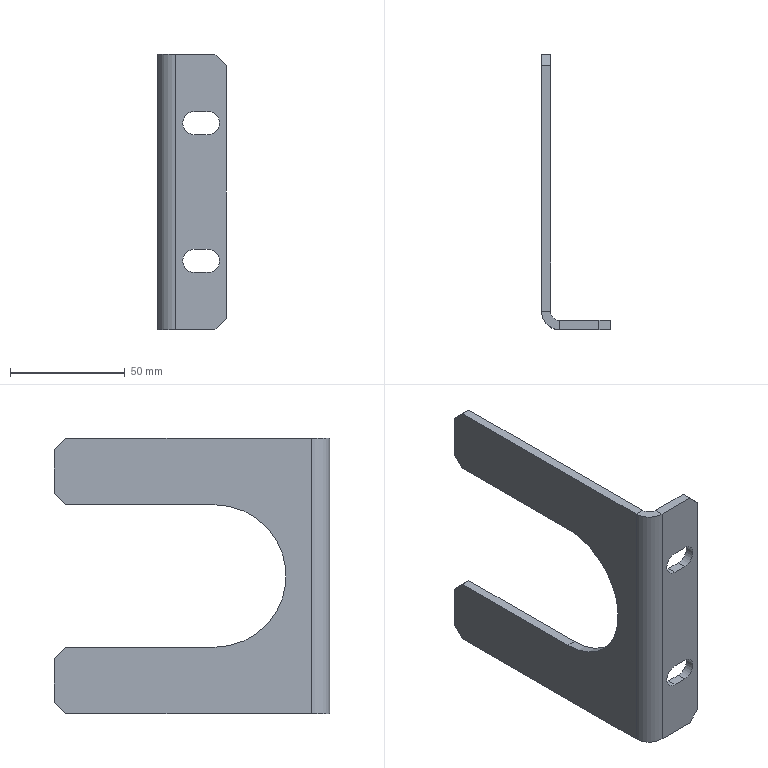Part | STEP file | 02 Bent plate | 1 solid | 32 faces | box 30 x 120 x 120 mm | volume 44037 mm3 | plane 25 | cylinder 7 | commonest cylinder face diameters 10 x4 8 x1 16 x1 62 x1